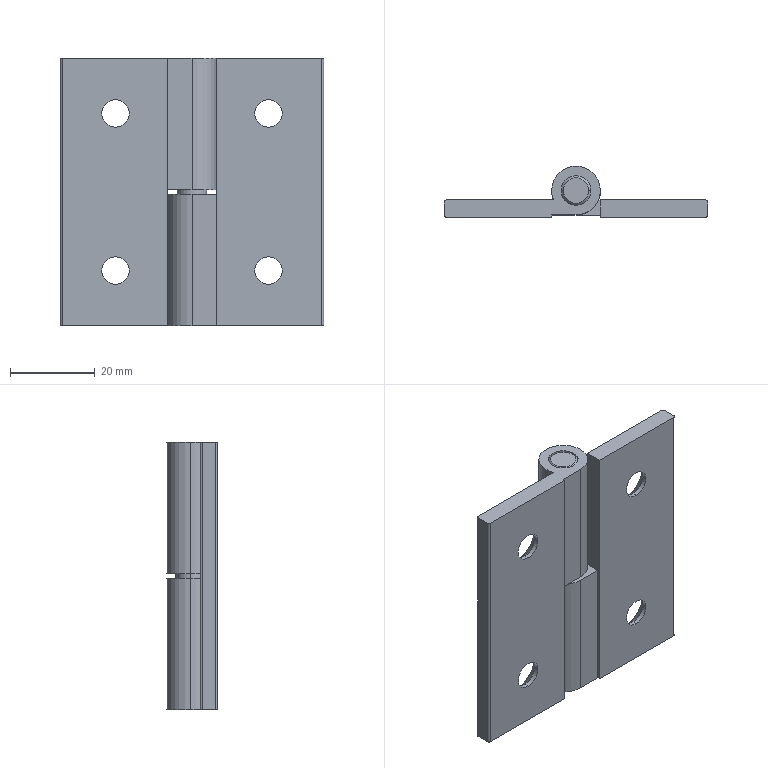Part | STEP file | Hinge assembly | 3 solids | 54 faces | box 62 x 12.05 x 63 mm | volume 18899 mm3 | cylinder 24 | plane 18 | cone 12 | commonest cylinder face diameters 6.5 x8 7 x6 11.5 x6 1 x4